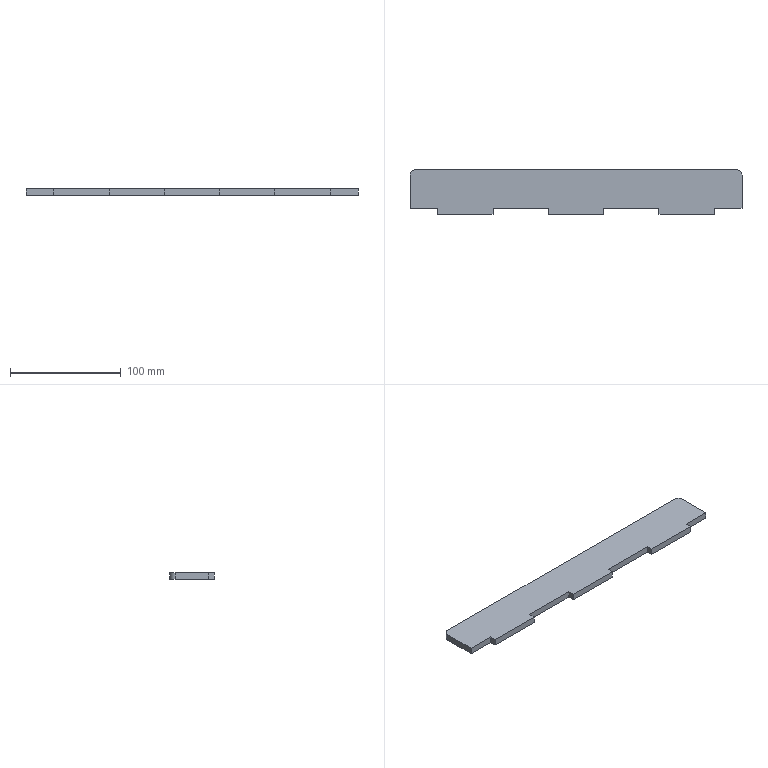Part | SolidWorks | features FlatPattern 1, SMBaseFlange 1, SheetMetal 1 | 1 solid | 20 faces | box 300 x 40.5 x 6 mm | volume 67886 mm3 | plane 18 | cylinder 2 | commonest cylinder face diameters 10 x2
STEP:
#1=CARTESIAN_POINT('',(117.463,-36.25,0.));
#2=VERTEX_POINT('',#1);
#3=CARTESIAN_POINT('',(117.463,-6.25,0.));
#4=VERTEX_POINT('',#3);
#5=CARTESIAN_POINT('',(117.463,-36.25,0.));
#6=DIRECTION('',(0.,1.,0.));
#7=VECTOR('',#6,1000.);
#8=LINE('',#5,#7);
#9=EDGE_CURVE('',#2,#4,#8,.T.);
#10=ORIENTED_EDGE('',*,*,#9,.F.);
#11=CARTESIAN_POINT('',(117.463,-36.25,-6.));
#12=VERTEX_POINT('',#11);
#13=CARTESIAN_POINT('',(117.463,-36.25,-6.));
#14=DIRECTION('',(0.,0.,1.));
#15=VECTOR('',#14,1000.);
#16=LINE('',#13,#15);
#17=EDGE_CURVE('',#12,#2,#16,.T.);
#18=ORIENTED_EDGE('',*,*,#17,.F.);
#19=CARTESIAN_POINT('',(117.463,-6.25,-6.));
#20=VERTEX_POINT('',#19);
#21=CARTESIAN_POINT('',(117.463,-36.25,-6.));
#22=DIRECTION('',(0.,1.,0.));
#23=VECTOR('',#22,1000.);
#24=LINE('',#21,#23);
#25=EDGE_CURVE('',#12,#20,#24,.T.);
#26=ORIENTED_EDGE('',*,*,#25,.T.);
#27=CARTESIAN_POINT('',(117.463,-6.25,-6.));
#28=DIRECTION('',(0.,0.,1.));
#29=VECTOR('',#28,1000.);
#30=LINE('',#27,#29);
#31=EDGE_CURVE('',#20,#4,#30,.T.);
#32=ORIENTED_EDGE('',*,*,#31,.T.);
#33=EDGE_LOOP('',(#10,#18,#26,#32));
#34=FACE_OUTER_BOUND('',#33,.T.);
#35=CARTESIAN_POINT('',(117.463,-36.25,-6.));
#36=DIRECTION('',(1.,0.,0.));
#37=DIRECTION('',(0.,0.,-1.));
#38=AXIS2_PLACEMENT_3D('',#35,#36,#37);
#39=PLANE('',#38);
#40=ADVANCED_FACE('',(#34),#39,.T.);
#41=CARTESIAN_POINT('',(92.463,-36.25,0.));
#42=VERTEX_POINT('',#41);
#43=CARTESIAN_POINT('',(117.463,-36.25,0.));
#44=DIRECTION('',(1.,0.,0.));
#45=VECTOR('',#44,1000.);
#46=LINE('',#43,#45);
#47=EDGE_CURVE('',#42,#2,#46,.T.);
#48=ORIENTED_EDGE('',*,*,#47,.F.);
#49=CARTESIAN_POINT('',(92.463,-36.25,-6.));
#50=VERTEX_POINT('',#49);
#51=CARTESIAN_POINT('',(92.463,-36.25,-6.));
#52=DIRECTION('',(0.,0.,1.));
#53=VECTOR('',#52,1000.);
#54=LINE('',#51,#53);
#55=EDGE_CURVE('',#50,#42,#54,.T.);
#56=ORIENTED_EDGE('',*,*,#55,.F.);
#57=CARTESIAN_POINT('',(117.463,-36.25,-6.));
#58=DIRECTION('',(1.,0.,0.));
#59=VECTOR('',#58,1000.);
#60=LINE('',#57,#59);
#61=EDGE_CURVE('',#50,#12,#60,.T.);
#62=ORIENTED_EDGE('',*,*,#61,.T.);
#63=ORIENTED_EDGE('',*,*,#17,.T.);
#64=EDGE_LOOP('',(#48,#56,#62,#63));
#65=FACE_OUTER_BOUND('',#64,.T.);
#66=CARTESIAN_POINT('',(117.463,-36.25,-6.));
#67=DIRECTION('',(0.,-1.,0.));
#68=DIRECTION('',(0.,0.,-1.));
#69=AXIS2_PLACEMENT_3D('',#66,#67,#68);
#70=PLANE('',#69);
#71=ADVANCED_FACE('',(#65),#70,.T.);
#72=CARTESIAN_POINT('',(92.463,-41.75,0.));
#73=VERTEX_POINT('',#72);
#74=CARTESIAN_POINT('',(92.463,-36.25,0.));
#75=DIRECTION('',(0.,1.,0.));
#76=VECTOR('',#75,1000.);
#77=LINE('',#74,#76);
#78=EDGE_CURVE('',#73,#42,#77,.T.);
#79=ORIENTED_EDGE('',*,*,#78,.F.);
#80=CARTESIAN_POINT('',(92.463,-41.75,-6.));
#81=VERTEX_POINT('',#80);
#82=CARTESIAN_POINT('',(92.463,-41.75,-6.));
#83=DIRECTION('',(0.,0.,1.));
#84=VECTOR('',#83,1000.);
#85=LINE('',#82,#84);
#86=EDGE_CURVE('',#81,#73,#85,.T.);
#87=ORIENTED_EDGE('',*,*,#86,.F.);
#88=CARTESIAN_POINT('',(92.463,-36.25,-6.));
#89=DIRECTION('',(0.,1.,0.));
#90=VECTOR('',#89,1000.);
#91=LINE('',#88,#90);
#92=EDGE_CURVE('',#81,#50,#91,.T.);
#93=ORIENTED_EDGE('',*,*,#92,.T.);
#94=ORIENTED_EDGE('',*,*,#55,.T.);
#95=EDGE_LOOP('',(#79,#87,#93,#94));
#96=FACE_OUTER_BOUND('',#95,.T.);
#97=CARTESIAN_POINT('',(92.463,-36.25,-6.));
#98=DIRECTION('',(1.,0.,0.));
#99=DIRECTION('',(0.,0.,-1.));
#100=AXIS2_PLACEMENT_3D('',#97,#98,#99);
#101=PLANE('',#100);
#102=ADVANCED_FACE('',(#96),#101,.T.);
#103=CARTESIAN_POINT('',(42.463,-41.75,0.));
#104=VERTEX_POINT('',#103);
#105=CARTESIAN_POINT('',(92.463,-41.75,0.));
#106=DIRECTION('',(1.,0.,0.));
#107=VECTOR('',#106,1000.);
#108=LINE('',#105,#107);
#109=EDGE_CURVE('',#104,#73,#108,.T.);
#110=ORIENTED_EDGE('',*,*,#109,.F.);
#111=CARTESIAN_POINT('',(42.463,-41.75,-6.));
#112=VERTEX_POINT('',#111);
#113=CARTESIAN_POINT('',(42.463,-41.75,-6.));
#114=DIRECTION('',(0.,0.,1.));
#115=VECTOR('',#114,1000.);
#116=LINE('',#113,#115);
#117=EDGE_CURVE('',#112,#104,#116,.T.);
#118=ORIENTED_EDGE('',*,*,#117,.F.);
#119=CARTESIAN_POINT('',(92.463,-41.75,-6.));
#120=DIRECTION('',(1.,0.,0.));
#121=VECTOR('',#120,1000.);
#122=LINE('',#119,#121);
#123=EDGE_CURVE('',#112,#81,#122,.T.);
#124=ORIENTED_EDGE('',*,*,#123,.T.);
#125=ORIENTED_EDGE('',*,*,#86,.T.);
#126=EDGE_LOOP('',(#110,#118,#124,#125));
#127=FACE_OUTER_BOUND('',#126,.T.);
#128=CARTESIAN_POINT('',(92.463,-41.75,-6.));
#129=DIRECTION('',(0.,-1.,0.));
#130=DIRECTION('',(1.,0.,0.));
#131=AXIS2_PLACEMENT_3D('',#128,#129,#130);
#132=PLANE('',#131);
#133=ADVANCED_FACE('',(#127),#132,.T.);
#134=CARTESIAN_POINT('',(42.463,-36.25,0.));
#135=VERTEX_POINT('',#134);
#136=CARTESIAN_POINT('',(42.463,-41.75,0.));
#137=DIRECTION('',(0.,-1.,0.));
#138=VECTOR('',#137,1000.);
#139=LINE('',#136,#138);
#140=EDGE_CURVE('',#135,#104,#139,.T.);
#141=ORIENTED_EDGE('',*,*,#140,.F.);
#142=CARTESIAN_POINT('',(42.463,-36.25,-6.));
#143=VERTEX_POINT('',#142);
#144=CARTESIAN_POINT('',(42.463,-36.25,-6.));
#145=DIRECTION('',(0.,0.,1.));
#146=VECTOR('',#145,1000.);
#147=LINE('',#144,#146);
#148=EDGE_CURVE('',#143,#135,#147,.T.);
#149=ORIENTED_EDGE('',*,*,#148,.F.);
#150=CARTESIAN_POINT('',(42.463,-41.75,-6.));
#151=DIRECTION('',(0.,-1.,0.));
#152=VECTOR('',#151,1000.);
#153=LINE('',#150,#152);
#154=EDGE_CURVE('',#143,#112,#153,.T.);
#155=ORIENTED_EDGE('',*,*,#154,.T.);
#156=ORIENTED_EDGE('',*,*,#117,.T.);
#157=EDGE_LOOP('',(#141,#149,#155,#156));
#158=FACE_OUTER_BOUND('',#157,.T.);
#159=CARTESIAN_POINT('',(42.463,-41.75,-6.));
#160=DIRECTION('',(-1.,0.,0.));
#161=DIRECTION('',(0.,0.,1.));
#162=AXIS2_PLACEMENT_3D('',#159,#160,#161);
#163=PLANE('',#162);
#164=ADVANCED_FACE('',(#158),#163,.T.);
#165=CARTESIAN_POINT('',(-7.537,-36.25,0.));
#166=VERTEX_POINT('',#165);
#167=CARTESIAN_POINT('',(42.463,-36.25,0.));
#168=DIRECTION('',(1.,0.,0.));
#169=VECTOR('',#168,1000.);
#170=LINE('',#167,#169);
#171=EDGE_CURVE('',#166,#135,#170,.T.);
#172=ORIENTED_EDGE('',*,*,#171,.F.);
#173=CARTESIAN_POINT('',(-7.537,-36.25,-6.));
#174=VERTEX_POINT('',#173);
#175=CARTESIAN_POINT('',(-7.537,-36.25,-6.));
#176=DIRECTION('',(0.,0.,1.));
#177=VECTOR('',#176,1000.);
#178=LINE('',#175,#177);
#179=EDGE_CURVE('',#174,#166,#178,.T.);
#180=ORIENTED_EDGE('',*,*,#179,.F.);
#181=CARTESIAN_POINT('',(42.463,-36.25,-6.));
#182=DIRECTION('',(1.,0.,0.));
#183=VECTOR('',#182,1000.);
#184=LINE('',#181,#183);
#185=EDGE_CURVE('',#174,#143,#184,.T.);
#186=ORIENTED_EDGE('',*,*,#185,.T.);
#187=ORIENTED_EDGE('',*,*,#148,.T.);
#188=EDGE_LOOP('',(#172,#180,#186,#187));
#189=FACE_OUTER_BOUND('',#188,.T.);
#190=CARTESIAN_POINT('',(42.463,-36.25,-6.));
#191=DIRECTION('',(0.,-1.,0.));
#192=DIRECTION('',(0.,0.,-1.));
#193=AXIS2_PLACEMENT_3D('',#190,#191,#192);
#194=PLANE('',#193);
#195=ADVANCED_FACE('',(#189),#194,.T.);
#196=CARTESIAN_POINT('',(-7.537,-41.75,0.));
#197=VERTEX_POINT('',#196);
#198=CARTESIAN_POINT('',(-7.537,-36.25,0.));
#199=DIRECTION('',(0.,1.,0.));
#200=VECTOR('',#199,1000.);
#201=LINE('',#198,#200);
#202=EDGE_CURVE('',#197,#166,#201,.T.);
#203=ORIENTED_EDGE('',*,*,#202,.F.);
#204=CARTESIAN_POINT('',(-7.537,-41.75,-6.));
#205=VERTEX_POINT('',#204);
#206=CARTESIAN_POINT('',(-7.537,-41.75,-6.));
#207=DIRECTION('',(0.,0.,1.));
#208=VECTOR('',#207,1000.);
#209=LINE('',#206,#208);
#210=EDGE_CURVE('',#205,#197,#209,.T.);
#211=ORIENTED_EDGE('',*,*,#210,.F.);
#212=CARTESIAN_POINT('',(-7.537,-36.25,-6.));
#213=DIRECTION('',(0.,1.,0.));
#214=VECTOR('',#213,1000.);
#215=LINE('',#212,#214);
#216=EDGE_CURVE('',#205,#174,#215,.T.);
#217=ORIENTED_EDGE('',*,*,#216,.T.);
#218=ORIENTED_EDGE('',*,*,#179,.T.);
#219=EDGE_LOOP('',(#203,#211,#217,#218));
#220=FACE_OUTER_BOUND('',#219,.T.);
#221=CARTESIAN_POINT('',(-7.537,-36.25,-6.));
#222=DIRECTION('',(1.,0.,0.));
#223=DIRECTION('',(0.,1.,0.));
#224=AXIS2_PLACEMENT_3D('',#221,#222,#223);
#225=PLANE('',#224);
#226=ADVANCED_FACE('',(#220),#225,.T.);
#227=CARTESIAN_POINT('',(-57.537,-41.75,0.));
#228=VERTEX_POINT('',#227);
#229=CARTESIAN_POINT('',(-7.537,-41.75,0.));
#230=DIRECTION('',(1.,0.,0.));
#231=VECTOR('',#230,1000.);
#232=LINE('',#229,#231);
#233=EDGE_CURVE('',#228,#197,#232,.T.);
#234=ORIENTED_EDGE('',*,*,#233,.F.);
#235=CARTESIAN_POINT('',(-57.537,-41.75,-6.));
#236=VERTEX_POINT('',#235);
#237=CARTESIAN_POINT('',(-57.537,-41.75,-6.));
#238=DIRECTION('',(0.,0.,1.));
#239=VECTOR('',#238,1000.);
#240=LINE('',#237,#239);
#241=EDGE_CURVE('',#236,#228,#240,.T.);
#242=ORIENTED_EDGE('',*,*,#241,.F.);
#243=CARTESIAN_POINT('',(-7.537,-41.75,-6.));
#244=DIRECTION('',(1.,0.,0.));
#245=VECTOR('',#244,1000.);
#246=LINE('',#243,#245);
#247=EDGE_CURVE('',#236,#205,#246,.T.);
#248=ORIENTED_EDGE('',*,*,#247,.T.);
#249=ORIENTED_EDGE('',*,*,#210,.T.);
#250=EDGE_LOOP('',(#234,#242,#248,#249));
#251=FACE_OUTER_BOUND('',#250,.T.);
#252=CARTESIAN_POINT('',(-7.537,-41.75,-6.));
#253=DIRECTION('',(0.,-1.,0.));
#254=DIRECTION('',(0.,0.,-1.));
#255=AXIS2_PLACEMENT_3D('',#252,#253,#254);
#256=PLANE('',#255);
#257=ADVANCED_FACE('',(#251),#256,.T.);
#258=CARTESIAN_POINT('',(-57.537,-36.25,0.));
#259=VERTEX_POINT('',#258);
#260=CARTESIAN_POINT('',(-57.537,-41.75,0.));
#261=DIRECTION('',(0.,-1.,0.));
#262=VECTOR('',#261,1000.);
#263=LINE('',#260,#262);
#264=EDGE_CURVE('',#259,#228,#263,.T.);
#265=ORIENTED_EDGE('',*,*,#264,.F.);
#266=CARTESIAN_POINT('',(-57.537,-36.25,-6.));
#267=VERTEX_POINT('',#266);
#268=CARTESIAN_POINT('',(-57.537,-36.25,-6.));
#269=DIRECTION('',(0.,0.,1.));
#270=VECTOR('',#269,1000.);
#271=LINE('',#268,#270);
#272=EDGE_CURVE('',#267,#259,#271,.T.);
#273=ORIENTED_EDGE('',*,*,#272,.F.);
#274=CARTESIAN_POINT('',(-57.537,-41.75,-6.));
#275=DIRECTION('',(0.,-1.,0.));
#276=VECTOR('',#275,1000.);
#277=LINE('',#274,#276);
#278=EDGE_CURVE('',#267,#236,#277,.T.);
#279=ORIENTED_EDGE('',*,*,#278,.T.);
#280=ORIENTED_EDGE('',*,*,#241,.T.);
#281=EDGE_LOOP('',(#265,#273,#279,#280));
#282=FACE_OUTER_BOUND('',#281,.T.);
#283=CARTESIAN_POINT('',(-57.537,-41.75,-6.));
#284=DIRECTION('',(-1.,0.,0.));
#285=DIRECTION('',(0.,0.,1.));
#286=AXIS2_PLACEMENT_3D('',#283,#284,#285);
#287=PLANE('',#286);
#288=ADVANCED_FACE('',(#282),#287,.T.);
#289=CARTESIAN_POINT('',(-107.537,-36.25,0.));
#290=VERTEX_POINT('',#289);
#291=CARTESIAN_POINT('',(-57.537,-36.25,0.));
#292=DIRECTION('',(1.,0.,0.));
#293=VECTOR('',#292,1000.);
#294=LINE('',#291,#293);
#295=EDGE_CURVE('',#290,#259,#294,.T.);
#296=ORIENTED_EDGE('',*,*,#295,.F.);
#297=CARTESIAN_POINT('',(-107.537,-36.25,-6.));
#298=VERTEX_POINT('',#297);
#299=CARTESIAN_POINT('',(-107.537,-36.25,-6.));
#300=DIRECTION('',(0.,0.,1.));
#301=VECTOR('',#300,1000.);
#302=LINE('',#299,#301);
#303=EDGE_CURVE('',#298,#290,#302,.T.);
#304=ORIENTED_EDGE('',*,*,#303,.F.);
#305=CARTESIAN_POINT('',(-57.537,-36.25,-6.));
#306=DIRECTION('',(1.,0.,0.));
#307=VECTOR('',#306,1000.);
#308=LINE('',#305,#307);
#309=EDGE_CURVE('',#298,#267,#308,.T.);
#310=ORIENTED_EDGE('',*,*,#309,.T.);
#311=ORIENTED_EDGE('',*,*,#272,.T.);
#312=EDGE_LOOP('',(#296,#304,#310,#311));
#313=FACE_OUTER_BOUND('',#312,.T.);
#314=CARTESIAN_POINT('',(-57.537,-36.25,-6.));
#315=DIRECTION('',(0.,-1.,0.));
#316=DIRECTION('',(1.,0.,0.));
#317=AXIS2_PLACEMENT_3D('',#314,#315,#316);
#318=PLANE('',#317);
#319=ADVANCED_FACE('',(#313),#318,.T.);
#320=CARTESIAN_POINT('',(-107.537,-41.75,0.));
#321=VERTEX_POINT('',#320);
#322=CARTESIAN_POINT('',(-107.537,-41.75,0.));
#323=DIRECTION('',(0.,1.,0.));
#324=VECTOR('',#323,1000.);
#325=LINE('',#322,#324);
#326=EDGE_CURVE('',#321,#290,#325,.T.);
#327=ORIENTED_EDGE('',*,*,#326,.F.);
#328=CARTESIAN_POINT('',(-107.537,-41.75,-6.));
#329=VERTEX_POINT('',#328);
#330=CARTESIAN_POINT('',(-107.537,-41.75,-6.));
#331=DIRECTION('',(0.,0.,1.));
#332=VECTOR('',#331,1000.);
#333=LINE('',#330,#332);
#334=EDGE_CURVE('',#329,#321,#333,.T.);
#335=ORIENTED_EDGE('',*,*,#334,.F.);
#336=CARTESIAN_POINT('',(-107.537,-41.75,-6.));
#337=DIRECTION('',(0.,1.,0.));
#338=VECTOR('',#337,1000.);
#339=LINE('',#336,#338);
#340=EDGE_CURVE('',#329,#298,#339,.T.);
#341=ORIENTED_EDGE('',*,*,#340,.T.);
#342=ORIENTED_EDGE('',*,*,#303,.T.);
#343=EDGE_LOOP('',(#327,#335,#341,#342));
#344=FACE_OUTER_BOUND('',#343,.T.);
#345=CARTESIAN_POINT('',(-107.537,-41.75,-6.));
#346=DIRECTION('',(1.,0.,0.));
#347=DIRECTION('',(0.,0.,-1.));
#348=AXIS2_PLACEMENT_3D('',#345,#346,#347);
#349=PLANE('',#348);
#350=ADVANCED_FACE('',(#344),#349,.T.);
#351=CARTESIAN_POINT('',(-157.537,-41.75,0.));
#352=VERTEX_POINT('',#351);
#353=CARTESIAN_POINT('',(-157.537,-41.75,0.));
#354=DIRECTION('',(1.,0.,0.));
#355=VECTOR('',#354,1000.);
#356=LINE('',#353,#355);
#357=EDGE_CURVE('',#352,#321,#356,.T.);
#358=ORIENTED_EDGE('',*,*,#357,.F.);
#359=CARTESIAN_POINT('',(-157.537,-41.75,-6.));
#360=VERTEX_POINT('',#359);
#361=CARTESIAN_POINT('',(-157.537,-41.75,-6.));
#362=DIRECTION('',(0.,0.,1.));
#363=VECTOR('',#362,1000.);
#364=LINE('',#361,#363);
#365=EDGE_CURVE('',#360,#352,#364,.T.);
#366=ORIENTED_EDGE('',*,*,#365,.F.);
#367=CARTESIAN_POINT('',(-157.537,-41.75,-6.));
#368=DIRECTION('',(1.,0.,0.));
#369=VECTOR('',#368,1000.);
#370=LINE('',#367,#369);
#371=EDGE_CURVE('',#360,#329,#370,.T.);
#372=ORIENTED_EDGE('',*,*,#371,.T.);
#373=ORIENTED_EDGE('',*,*,#334,.T.);
#374=EDGE_LOOP('',(#358,#366,#372,#373));
#375=FACE_OUTER_BOUND('',#374,.T.);
#376=CARTESIAN_POINT('',(-157.537,-41.75,-6.));
#377=DIRECTION('',(0.,-1.,0.));
#378=DIRECTION('',(0.,0.,-1.));
#379=AXIS2_PLACEMENT_3D('',#376,#377,#378);
#380=PLANE('',#379);
#381=ADVANCED_FACE('',(#375),#380,.T.);
#382=CARTESIAN_POINT('',(-157.537,-36.25,0.));
#383=VERTEX_POINT('',#382);
#384=CARTESIAN_POINT('',(-157.537,-36.25,0.));
#385=DIRECTION('',(0.,-1.,0.));
#386=VECTOR('',#385,1000.);
#387=LINE('',#384,#386);
#388=EDGE_CURVE('',#383,#352,#387,.T.);
#389=ORIENTED_EDGE('',*,*,#388,.F.);
#390=CARTESIAN_POINT('',(-157.537,-36.25,-6.));
#391=VERTEX_POINT('',#390);
#392=CARTESIAN_POINT('',(-157.537,-36.25,-6.));
#393=DIRECTION('',(0.,0.,1.));
#394=VECTOR('',#393,1000.);
#395=LINE('',#392,#394);
#396=EDGE_CURVE('',#391,#383,#395,.T.);
#397=ORIENTED_EDGE('',*,*,#396,.F.);
#398=CARTESIAN_POINT('',(-157.537,-36.25,-6.));
#399=DIRECTION('',(0.,-1.,0.));
#400=VECTOR('',#399,1000.);
#401=LINE('',#398,#400);
#402=EDGE_CURVE('',#391,#360,#401,.T.);
#403=ORIENTED_EDGE('',*,*,#402,.T.);
#404=ORIENTED_EDGE('',*,*,#365,.T.);
#405=EDGE_LOOP('',(#389,#397,#403,#404));
#406=FACE_OUTER_BOUND('',#405,.T.);
#407=CARTESIAN_POINT('',(-157.537,-36.25,-6.));
#408=DIRECTION('',(-1.,0.,0.));
#409=DIRECTION('',(0.,0.,1.));
#410=AXIS2_PLACEMENT_3D('',#407,#408,#409);
#411=PLANE('',#410);
#412=ADVANCED_FACE('',(#406),#411,.T.);
#413=CARTESIAN_POINT('',(-182.537,-36.25,0.));
#414=VERTEX_POINT('',#413);
#415=CARTESIAN_POINT('',(-157.537,-36.25,0.));
#416=DIRECTION('',(1.,0.,0.));
#417=VECTOR('',#416,1000.);
#418=LINE('',#415,#417);
#419=EDGE_CURVE('',#414,#383,#418,.T.);
#420=ORIENTED_EDGE('',*,*,#419,.F.);
#421=CARTESIAN_POINT('',(-182.537,-36.25,-6.));
#422=VERTEX_POINT('',#421);
#423=CARTESIAN_POINT('',(-182.537,-36.25,-6.));
#424=DIRECTION('',(0.,0.,1.));
#425=VECTOR('',#424,1000.);
#426=LINE('',#423,#425);
#427=EDGE_CURVE('',#422,#414,#426,.T.);
#428=ORIENTED_EDGE('',*,*,#427,.F.);
#429=CARTESIAN_POINT('',(-157.537,-36.25,-6.));
#430=DIRECTION('',(1.,0.,0.));
#431=VECTOR('',#430,1000.);
#432=LINE('',#429,#431);
#433=EDGE_CURVE('',#422,#391,#432,.T.);
#434=ORIENTED_EDGE('',*,*,#433,.T.);
#435=ORIENTED_EDGE('',*,*,#396,.T.);
#436=EDGE_LOOP('',(#420,#428,#434,#435));
#437=FACE_OUTER_BOUND('',#436,.T.);
#438=CARTESIAN_POINT('',(-157.537,-36.25,-6.));
#439=DIRECTION('',(0.,-1.,0.));
#440=DIRECTION('',(1.,0.,0.));
#441=AXIS2_PLACEMENT_3D('',#438,#439,#440);
#442=PLANE('',#441);
#443=ADVANCED_FACE('',(#437),#442,.T.);
#444=CARTESIAN_POINT('',(-182.537,-6.25,0.));
#445=VERTEX_POINT('',#444);
#446=CARTESIAN_POINT('',(-182.537,-36.25,0.));
#447=DIRECTION('',(0.,-1.,0.));
#448=VECTOR('',#447,1000.);
#449=LINE('',#446,#448);
#450=EDGE_CURVE('',#445,#414,#449,.T.);
#451=ORIENTED_EDGE('',*,*,#450,.F.);
#452=CARTESIAN_POINT('',(-182.537,-6.25,-6.));
#453=VERTEX_POINT('',#452);
#454=CARTESIAN_POINT('',(-182.537,-6.25,-6.));
#455=DIRECTION('',(0.,0.,1.));
#456=VECTOR('',#455,1000.);
#457=LINE('',#454,#456);
#458=EDGE_CURVE('',#453,#445,#457,.T.);
#459=ORIENTED_EDGE('',*,*,#458,.F.);
#460=CARTESIAN_POINT('',(-182.537,-36.25,-6.));
#461=DIRECTION('',(0.,-1.,0.));
#462=VECTOR('',#461,1000.);
#463=LINE('',#460,#462);
#464=EDGE_CURVE('',#453,#422,#463,.T.);
#465=ORIENTED_EDGE('',*,*,#464,.T.);
#466=ORIENTED_EDGE('',*,*,#427,.T.);
#467=EDGE_LOOP('',(#451,#459,#465,#466));
#468=FACE_OUTER_BOUND('',#467,.T.);
#469=CARTESIAN_POINT('',(-182.537,-36.25,-6.));
#470=DIRECTION('',(-1.,0.,0.));
#471=DIRECTION('',(0.,0.,1.));
#472=AXIS2_PLACEMENT_3D('',#469,#470,#471);
#473=PLANE('',#472);
#474=ADVANCED_FACE('',(#468),#473,.T.);
#475=CARTESIAN_POINT('',(-177.537,-1.25,0.));
#476=VERTEX_POINT('',#475);
#477=CARTESIAN_POINT('',(-177.537,-6.25,0.));
#478=DIRECTION('',(0.,0.,1.));
#479=DIRECTION('',(1.,0.,0.));
#480=AXIS2_PLACEMENT_3D('',#477,#478,#479);
#481=CIRCLE('',#480,5.);
#482=EDGE_CURVE('',#476,#445,#481,.T.);
#483=ORIENTED_EDGE('',*,*,#482,.F.);
#484=CARTESIAN_POINT('',(-177.537,-1.25,-6.));
#485=VERTEX_POINT('',#484);
#486=CARTESIAN_POINT('',(-177.537,-1.25,-6.));
#487=DIRECTION('',(0.,0.,1.));
#488=VECTOR('',#487,1000.);
#489=LINE('',#486,#488);
#490=EDGE_CURVE('',#485,#476,#489,.T.);
#491=ORIENTED_EDGE('',*,*,#490,.F.);
#492=CARTESIAN_POINT('',(-177.537,-6.25,-6.));
#493=DIRECTION('',(0.,0.,1.));
#494=DIRECTION('',(1.,0.,0.));
#495=AXIS2_PLACEMENT_3D('',#492,#493,#494);
#496=CIRCLE('',#495,5.);
#497=EDGE_CURVE('',#485,#453,#496,.T.);
#498=ORIENTED_EDGE('',*,*,#497,.T.);
#499=ORIENTED_EDGE('',*,*,#458,.T.);
#500=EDGE_LOOP('',(#483,#491,#498,#499));
#501=FACE_OUTER_BOUND('',#500,.T.);
#502=CARTESIAN_POINT('',(-177.537,-6.25,-6.));
#503=DIRECTION('',(0.,0.,1.));
#504=DIRECTION('',(1.,0.,0.));
#505=AXIS2_PLACEMENT_3D('',#502,#503,#504);
#506=CYLINDRICAL_SURFACE('',#505,5.);
#507=ADVANCED_FACE('',(#501),#506,.T.);
#508=CARTESIAN_POINT('',(112.463,-1.25,0.));
#509=VERTEX_POINT('',#508);
#510=CARTESIAN_POINT('',(112.463,-1.25,0.));
#511=DIRECTION('',(-1.,0.,0.));
#512=VECTOR('',#511,1000.);
#513=LINE('',#510,#512);
#514=EDGE_CURVE('',#509,#476,#513,.T.);
#515=ORIENTED_EDGE('',*,*,#514,.F.);
#516=CARTESIAN_POINT('',(112.463,-1.25,-6.));
#517=VERTEX_POINT('',#516);
#518=CARTESIAN_POINT('',(112.463,-1.25,-6.));
#519=DIRECTION('',(0.,0.,1.));
#520=VECTOR('',#519,1000.);
#521=LINE('',#518,#520);
#522=EDGE_CURVE('',#517,#509,#521,.T.);
#523=ORIENTED_EDGE('',*,*,#522,.F.);
#524=CARTESIAN_POINT('',(112.463,-1.25,-6.));
#525=DIRECTION('',(-1.,0.,0.));
#526=VECTOR('',#525,1000.);
#527=LINE('',#524,#526);
#528=EDGE_CURVE('',#517,#485,#527,.T.);
#529=ORIENTED_EDGE('',*,*,#528,.T.);
#530=ORIENTED_EDGE('',*,*,#490,.T.);
#531=EDGE_LOOP('',(#515,#523,#529,#530));
#532=FACE_OUTER_BOUND('',#531,.T.);
#533=CARTESIAN_POINT('',(112.463,-1.25,-6.));
#534=DIRECTION('',(0.,1.,0.));
#535=DIRECTION('',(-1.,0.,0.));
#536=AXIS2_PLACEMENT_3D('',#533,#534,#535);
#537=PLANE('',#536);
#538=ADVANCED_FACE('',(#532),#537,.T.);
#539=CARTESIAN_POINT('',(112.463,-6.25,0.));
#540=DIRECTION('',(0.,0.,1.));
#541=DIRECTION('',(1.,0.,0.));
#542=AXIS2_PLACEMENT_3D('',#539,#540,#541);
#543=CIRCLE('',#542,5.);
#544=EDGE_CURVE('',#4,#509,#543,.T.);
#545=ORIENTED_EDGE('',*,*,#544,.F.);
#546=ORIENTED_EDGE('',*,*,#31,.F.);
#547=CARTESIAN_POINT('',(112.463,-6.25,-6.));
#548=DIRECTION('',(0.,0.,1.));
#549=DIRECTION('',(1.,0.,0.));
#550=AXIS2_PLACEMENT_3D('',#547,#548,#549);
#551=CIRCLE('',#550,5.);
#552=EDGE_CURVE('',#20,#517,#551,.T.);
#553=ORIENTED_EDGE('',*,*,#552,.T.);
#554=ORIENTED_EDGE('',*,*,#522,.T.);
#555=EDGE_LOOP('',(#545,#546,#553,#554));
#556=FACE_OUTER_BOUND('',#555,.T.);
#557=CARTESIAN_POINT('',(112.463,-6.25,-6.));
#558=DIRECTION('',(0.,0.,1.));
#559=DIRECTION('',(1.,0.,0.));
#560=AXIS2_PLACEMENT_3D('',#557,#558,#559);
#561=CYLINDRICAL_SURFACE('',#560,5.);
#562=ADVANCED_FACE('',(#556),#561,.T.);
#563=ORIENTED_EDGE('',*,*,#25,.F.);
#564=ORIENTED_EDGE('',*,*,#61,.F.);
#565=ORIENTED_EDGE('',*,*,#92,.F.);
#566=ORIENTED_EDGE('',*,*,#123,.F.);
#567=ORIENTED_EDGE('',*,*,#154,.F.);
#568=ORIENTED_EDGE('',*,*,#185,.F.);
#569=ORIENTED_EDGE('',*,*,#216,.F.);
#570=ORIENTED_EDGE('',*,*,#247,.F.);
#571=ORIENTED_EDGE('',*,*,#278,.F.);
#572=ORIENTED_EDGE('',*,*,#309,.F.);
#573=ORIENTED_EDGE('',*,*,#340,.F.);
#574=ORIENTED_EDGE('',*,*,#371,.F.);
#575=ORIENTED_EDGE('',*,*,#402,.F.);
#576=ORIENTED_EDGE('',*,*,#433,.F.);
#577=ORIENTED_EDGE('',*,*,#464,.F.);
#578=ORIENTED_EDGE('',*,*,#497,.F.);
#579=ORIENTED_EDGE('',*,*,#528,.F.);
#580=ORIENTED_EDGE('',*,*,#552,.F.);
#581=EDGE_LOOP('',(#563,#564,#565,#566,#567,#568,#569,#570,#571,#572,#573,#574,#575,#576,#577,#578,#579,#580));
#582=FACE_OUTER_BOUND('',#581,.T.);
#583=CARTESIAN_POINT('',(112.463,-6.25,-6.));
#584=DIRECTION('',(0.,0.,1.));
#585=DIRECTION('',(1.,0.,0.));
#586=AXIS2_PLACEMENT_3D('',#583,#584,#585);
#587=PLANE('',#586);
#588=ADVANCED_FACE('',(#582),#587,.F.);
#589=ORIENTED_EDGE('',*,*,#9,.T.);
#590=ORIENTED_EDGE('',*,*,#544,.T.);
#591=ORIENTED_EDGE('',*,*,#514,.T.);
#592=ORIENTED_EDGE('',*,*,#482,.T.);
#593=ORIENTED_EDGE('',*,*,#450,.T.);
#594=ORIENTED_EDGE('',*,*,#419,.T.);
#595=ORIENTED_EDGE('',*,*,#388,.T.);
#596=ORIENTED_EDGE('',*,*,#357,.T.);
#597=ORIENTED_EDGE('',*,*,#326,.T.);
#598=ORIENTED_EDGE('',*,*,#295,.T.);
#599=ORIENTED_EDGE('',*,*,#264,.T.);
#600=ORIENTED_EDGE('',*,*,#233,.T.);
#601=ORIENTED_EDGE('',*,*,#202,.T.);
#602=ORIENTED_EDGE('',*,*,#171,.T.);
#603=ORIENTED_EDGE('',*,*,#140,.T.);
#604=ORIENTED_EDGE('',*,*,#109,.T.);
#605=ORIENTED_EDGE('',*,*,#78,.T.);
#606=ORIENTED_EDGE('',*,*,#47,.T.);
#607=EDGE_LOOP('',(#589,#590,#591,#592,#593,#594,#595,#596,#597,#598,#599,#600,#601,#602,#603,#604,#605,#606));
#608=FACE_OUTER_BOUND('',#607,.T.);
#609=CARTESIAN_POINT('',(112.463,-6.25,0.));
#610=DIRECTION('',(0.,0.,1.));
#611=DIRECTION('',(1.,0.,0.));
#612=AXIS2_PLACEMENT_3D('',#609,#610,#611);
#613=PLANE('',#612);
#614=ADVANCED_FACE('',(#608),#613,.T.);
#615=CLOSED_SHELL('',(#40,#71,#102,#133,#164,#195,#226,#257,#288,#319,#350,#381,#412,#443,#474,#507,#538,#562,#588,#614));
#616=MANIFOLD_SOLID_BREP('',#615);
#617=CARTESIAN_POINT('',(0.,0.,0.));
#618=DIRECTION('',(0.,0.,1.));
#619=DIRECTION('',(1.,0.,0.));
#620=AXIS2_PLACEMENT_3D('',#617,#618,#619);
#621=(LENGTH_UNIT()NAMED_UNIT(*)SI_UNIT(.MILLI.,.METRE.));
#622=UNCERTAINTY_MEASURE_WITH_UNIT(LENGTH_MEASURE(0.00001),#621,'','');
#623=(NAMED_UNIT(*)PLANE_ANGLE_UNIT()SI_UNIT($,.RADIAN.));
#624=(NAMED_UNIT(*)SI_UNIT($,.STERADIAN.)SOLID_ANGLE_UNIT());
#625=(GEOMETRIC_REPRESENTATION_CONTEXT(3)GLOBAL_UNCERTAINTY_ASSIGNED_CONTEXT((#622))GLOBAL_UNIT_ASSIGNED_CONTEXT((#621,#623,#624))REPRESENTATION_CONTEXT('',''));
#626=ADVANCED_BREP_SHAPE_REPRESENTATION('',(#616,#620),#625);